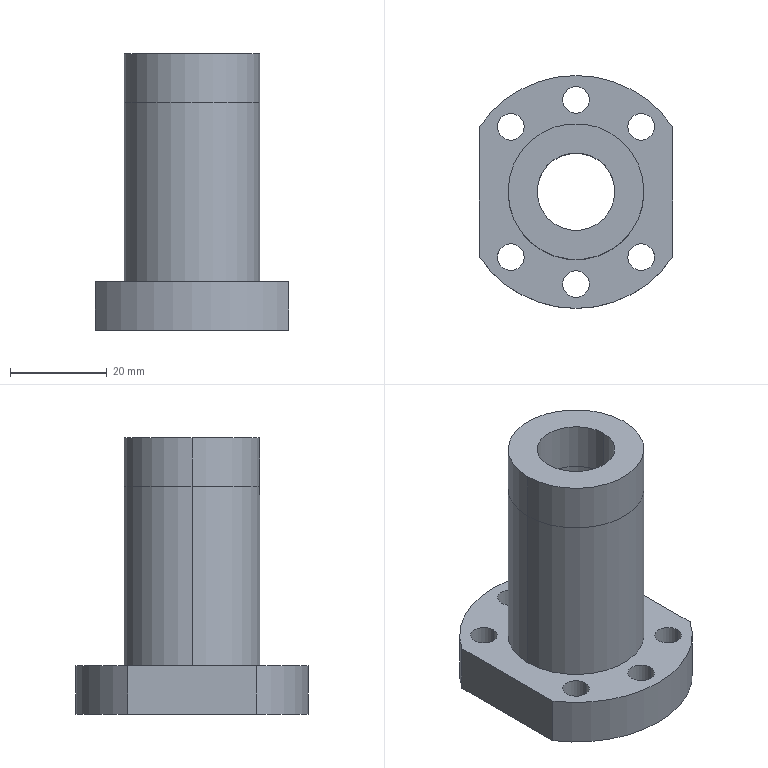Part | SolidWorks | features Extrusion 1, HoleWzd 1, ICE 1, MirrorPattern 1, Split 1 | 3 solids | 32 faces | box 40 x 48 x 57 mm | volume 32709 mm3 | cylinder 24 | plane 8 | commonest cylinder face diameters 5.5 x12 16 x6 28 x4 48 x2
STEP:
#1=CARTESIAN_POINT('',(-8.,0.,47.));
#2=VERTEX_POINT('',#1);
#3=CARTESIAN_POINT('',(8.,0.,47.));
#4=VERTEX_POINT('',#3);
#5=CARTESIAN_POINT('',(0.,0.,47.));
#6=DIRECTION('',(0.,0.,1.));
#7=DIRECTION('',(1.,0.,0.));
#8=AXIS2_PLACEMENT_3D('',#5,#6,#7);
#9=CIRCLE('',#8,8.);
#10=EDGE_CURVE('',#2,#4,#9,.T.);
#11=ORIENTED_EDGE('',*,*,#10,.T.);
#12=CARTESIAN_POINT('',(8.,0.,10.));
#13=VERTEX_POINT('',#12);
#14=CARTESIAN_POINT('',(8.,0.,57.));
#15=DIRECTION('',(0.,0.,-1.));
#16=VECTOR('',#15,1000.);
#17=LINE('',#14,#16);
#18=EDGE_CURVE('',#4,#13,#17,.T.);
#19=ORIENTED_EDGE('',*,*,#18,.T.);
#20=CARTESIAN_POINT('',(-8.,0.,10.));
#21=VERTEX_POINT('',#20);
#22=CARTESIAN_POINT('',(0.,0.,10.));
#23=DIRECTION('',(0.,0.,-1.));
#24=DIRECTION('',(-1.,0.,0.));
#25=AXIS2_PLACEMENT_3D('',#22,#23,#24);
#26=CIRCLE('',#25,8.);
#27=EDGE_CURVE('',#13,#21,#26,.T.);
#28=ORIENTED_EDGE('',*,*,#27,.T.);
#29=CARTESIAN_POINT('',(-8.,0.,57.));
#30=DIRECTION('',(0.,0.,-1.));
#31=VECTOR('',#30,1000.);
#32=LINE('',#29,#31);
#33=EDGE_CURVE('',#2,#21,#32,.T.);
#34=ORIENTED_EDGE('',*,*,#33,.F.);
#35=EDGE_LOOP('',(#11,#19,#28,#34));
#36=FACE_OUTER_BOUND('',#35,.T.);
#37=CARTESIAN_POINT('',(0.,0.,57.));
#38=DIRECTION('',(0.,0.,-1.));
#39=DIRECTION('',(-1.,0.,0.));
#40=AXIS2_PLACEMENT_3D('',#37,#38,#39);
#41=CYLINDRICAL_SURFACE('',#40,8.);
#42=ADVANCED_FACE('',(#36),#41,.F.);
#43=CARTESIAN_POINT('',(14.,0.,47.));
#44=VERTEX_POINT('',#43);
#45=CARTESIAN_POINT('',(-14.,0.,47.));
#46=VERTEX_POINT('',#45);
#47=CARTESIAN_POINT('',(0.,0.,47.));
#48=DIRECTION('',(0.,0.,1.));
#49=DIRECTION('',(1.,0.,0.));
#50=AXIS2_PLACEMENT_3D('',#47,#48,#49);
#51=CIRCLE('',#50,14.);
#52=EDGE_CURVE('',#44,#46,#51,.T.);
#53=ORIENTED_EDGE('',*,*,#52,.F.);
#54=CARTESIAN_POINT('',(14.,0.,10.));
#55=VERTEX_POINT('',#54);
#56=CARTESIAN_POINT('',(14.,0.,57.));
#57=DIRECTION('',(0.,0.,-1.));
#58=VECTOR('',#57,1000.);
#59=LINE('',#56,#58);
#60=EDGE_CURVE('',#44,#55,#59,.T.);
#61=ORIENTED_EDGE('',*,*,#60,.T.);
#62=CARTESIAN_POINT('',(-14.,0.,10.));
#63=VERTEX_POINT('',#62);
#64=CARTESIAN_POINT('',(0.,0.,10.));
#65=DIRECTION('',(0.,0.,-1.));
#66=DIRECTION('',(-1.,0.,0.));
#67=AXIS2_PLACEMENT_3D('',#64,#65,#66);
#68=CIRCLE('',#67,14.);
#69=EDGE_CURVE('',#63,#55,#68,.T.);
#70=ORIENTED_EDGE('',*,*,#69,.F.);
#71=CARTESIAN_POINT('',(-14.,0.,57.));
#72=DIRECTION('',(0.,0.,-1.));
#73=VECTOR('',#72,1000.);
#74=LINE('',#71,#73);
#75=EDGE_CURVE('',#46,#63,#74,.T.);
#76=ORIENTED_EDGE('',*,*,#75,.F.);
#77=EDGE_LOOP('',(#53,#61,#70,#76));
#78=FACE_OUTER_BOUND('',#77,.T.);
#79=CARTESIAN_POINT('',(0.,0.,57.));
#80=DIRECTION('',(0.,0.,-1.));
#81=DIRECTION('',(-1.,0.,0.));
#82=AXIS2_PLACEMENT_3D('',#79,#80,#81);
#83=CYLINDRICAL_SURFACE('',#82,14.);
#84=ADVANCED_FACE('',(#78),#83,.T.);
#85=ORIENTED_EDGE('',*,*,#60,.F.);
#86=CARTESIAN_POINT('',(0.,0.,47.));
#87=DIRECTION('',(0.,0.,1.));
#88=DIRECTION('',(1.,0.,0.));
#89=AXIS2_PLACEMENT_3D('',#86,#87,#88);
#90=CIRCLE('',#89,14.);
#91=EDGE_CURVE('',#46,#44,#90,.T.);
#92=ORIENTED_EDGE('',*,*,#91,.F.);
#93=ORIENTED_EDGE('',*,*,#75,.T.);
#94=CARTESIAN_POINT('',(0.,0.,10.));
#95=DIRECTION('',(0.,0.,-1.));
#96=DIRECTION('',(-1.,0.,0.));
#97=AXIS2_PLACEMENT_3D('',#94,#95,#96);
#98=CIRCLE('',#97,14.);
#99=EDGE_CURVE('',#55,#63,#98,.T.);
#100=ORIENTED_EDGE('',*,*,#99,.F.);
#101=EDGE_LOOP('',(#85,#92,#93,#100));
#102=FACE_OUTER_BOUND('',#101,.T.);
#103=CARTESIAN_POINT('',(0.,0.,57.));
#104=DIRECTION('',(0.,0.,-1.));
#105=DIRECTION('',(-1.,0.,0.));
#106=AXIS2_PLACEMENT_3D('',#103,#104,#105);
#107=CYLINDRICAL_SURFACE('',#106,14.);
#108=ADVANCED_FACE('',(#102),#107,.T.);
#109=ORIENTED_EDGE('',*,*,#18,.F.);
#110=CARTESIAN_POINT('',(0.,0.,47.));
#111=DIRECTION('',(0.,0.,1.));
#112=DIRECTION('',(1.,0.,0.));
#113=AXIS2_PLACEMENT_3D('',#110,#111,#112);
#114=CIRCLE('',#113,8.);
#115=EDGE_CURVE('',#4,#2,#114,.T.);
#116=ORIENTED_EDGE('',*,*,#115,.T.);
#117=ORIENTED_EDGE('',*,*,#33,.T.);
#118=CARTESIAN_POINT('',(0.,0.,10.));
#119=DIRECTION('',(0.,0.,-1.));
#120=DIRECTION('',(-1.,0.,0.));
#121=AXIS2_PLACEMENT_3D('',#118,#119,#120);
#122=CIRCLE('',#121,8.);
#123=EDGE_CURVE('',#21,#13,#122,.T.);
#124=ORIENTED_EDGE('',*,*,#123,.T.);
#125=EDGE_LOOP('',(#109,#116,#117,#124));
#126=FACE_OUTER_BOUND('',#125,.T.);
#127=CARTESIAN_POINT('',(0.,0.,57.));
#128=DIRECTION('',(0.,0.,-1.));
#129=DIRECTION('',(-1.,0.,0.));
#130=AXIS2_PLACEMENT_3D('',#127,#128,#129);
#131=CYLINDRICAL_SURFACE('',#130,8.);
#132=ADVANCED_FACE('',(#126),#131,.F.);
#133=ORIENTED_EDGE('',*,*,#91,.T.);
#134=ORIENTED_EDGE('',*,*,#52,.T.);
#135=EDGE_LOOP('',(#133,#134));
#136=FACE_OUTER_BOUND('',#135,.T.);
#137=ORIENTED_EDGE('',*,*,#10,.F.);
#138=ORIENTED_EDGE('',*,*,#115,.F.);
#139=EDGE_LOOP('',(#137,#138));
#140=FACE_BOUND('',#139,.T.);
#141=CARTESIAN_POINT('',(-26.149,-24.01,47.));
#142=DIRECTION('',(0.,0.,1.));
#143=DIRECTION('',(1.,0.,0.));
#144=AXIS2_PLACEMENT_3D('',#141,#142,#143);
#145=PLANE('',#144);
#146=ADVANCED_FACE('',(#136,#140),#145,.T.);
#147=ORIENTED_EDGE('',*,*,#69,.T.);
#148=ORIENTED_EDGE('',*,*,#99,.T.);
#149=EDGE_LOOP('',(#147,#148));
#150=FACE_OUTER_BOUND('',#149,.T.);
#151=ORIENTED_EDGE('',*,*,#123,.F.);
#152=ORIENTED_EDGE('',*,*,#27,.F.);
#153=EDGE_LOOP('',(#151,#152));
#154=FACE_BOUND('',#153,.T.);
#155=CARTESIAN_POINT('',(-26.149,-24.01,10.));
#156=DIRECTION('',(0.,0.,-1.));
#157=DIRECTION('',(-1.,0.,0.));
#158=AXIS2_PLACEMENT_3D('',#155,#156,#157);
#159=PLANE('',#158);
#160=ADVANCED_FACE('',(#150,#154),#159,.T.);
#161=CLOSED_SHELL('',(#42,#84,#108,#132,#146,#160));
#162=MANIFOLD_SOLID_BREP('',#161);
#163=CARTESIAN_POINT('',(8.,0.,10.));
#164=VERTEX_POINT('',#163);
#165=CARTESIAN_POINT('',(-8.,0.,10.));
#166=VERTEX_POINT('',#165);
#167=CARTESIAN_POINT('',(0.,0.,10.));
#168=DIRECTION('',(0.,0.,-1.));
#169=DIRECTION('',(-1.,0.,0.));
#170=AXIS2_PLACEMENT_3D('',#167,#168,#169);
#171=CIRCLE('',#170,8.);
#172=EDGE_CURVE('',#164,#166,#171,.T.);
#173=ORIENTED_EDGE('',*,*,#172,.F.);
#174=CARTESIAN_POINT('',(8.,0.,0.));
#175=VERTEX_POINT('',#174);
#176=CARTESIAN_POINT('',(8.,0.,57.));
#177=DIRECTION('',(0.,0.,-1.));
#178=VECTOR('',#177,1000.);
#179=LINE('',#176,#178);
#180=EDGE_CURVE('',#164,#175,#179,.T.);
#181=ORIENTED_EDGE('',*,*,#180,.T.);
#182=CARTESIAN_POINT('',(-8.,0.,0.));
#183=VERTEX_POINT('',#182);
#184=CARTESIAN_POINT('',(0.,0.,0.));
#185=DIRECTION('',(0.,0.,1.));
#186=DIRECTION('',(1.,0.,0.));
#187=AXIS2_PLACEMENT_3D('',#184,#185,#186);
#188=CIRCLE('',#187,8.);
#189=EDGE_CURVE('',#183,#175,#188,.T.);
#190=ORIENTED_EDGE('',*,*,#189,.F.);
#191=CARTESIAN_POINT('',(-8.,0.,57.));
#192=DIRECTION('',(0.,0.,-1.));
#193=VECTOR('',#192,1000.);
#194=LINE('',#191,#193);
#195=EDGE_CURVE('',#166,#183,#194,.T.);
#196=ORIENTED_EDGE('',*,*,#195,.F.);
#197=EDGE_LOOP('',(#173,#181,#190,#196));
#198=FACE_OUTER_BOUND('',#197,.T.);
#199=CARTESIAN_POINT('',(0.,0.,57.));
#200=DIRECTION('',(0.,0.,-1.));
#201=DIRECTION('',(-1.,0.,0.));
#202=AXIS2_PLACEMENT_3D('',#199,#200,#201);
#203=CYLINDRICAL_SURFACE('',#202,8.);
#204=ADVANCED_FACE('',(#198),#203,.F.);
#205=CARTESIAN_POINT('',(-10.685,13.435,10.));
#206=VERTEX_POINT('',#205);
#207=CARTESIAN_POINT('',(-16.185,13.435,10.));
#208=VERTEX_POINT('',#207);
#209=CARTESIAN_POINT('',(-13.435,13.435,10.));
#210=DIRECTION('',(0.,0.,-1.));
#211=DIRECTION('',(-1.,0.,0.));
#212=AXIS2_PLACEMENT_3D('',#209,#210,#211);
#213=CIRCLE('',#212,2.75);
#214=EDGE_CURVE('',#206,#208,#213,.T.);
#215=ORIENTED_EDGE('',*,*,#214,.F.);
#216=CARTESIAN_POINT('',(-10.685,13.435,0.));
#217=VERTEX_POINT('',#216);
#218=CARTESIAN_POINT('',(-10.685,13.435,0.));
#219=DIRECTION('',(0.,0.,-1.));
#220=VECTOR('',#219,1000.);
#221=LINE('',#218,#220);
#222=EDGE_CURVE('',#206,#217,#221,.T.);
#223=ORIENTED_EDGE('',*,*,#222,.T.);
#224=CARTESIAN_POINT('',(-16.185,13.435,0.));
#225=VERTEX_POINT('',#224);
#226=CARTESIAN_POINT('',(-13.435,13.435,0.));
#227=DIRECTION('',(0.,0.,-1.));
#228=DIRECTION('',(-1.,0.,0.));
#229=AXIS2_PLACEMENT_3D('',#226,#227,#228);
#230=CIRCLE('',#229,2.75);
#231=EDGE_CURVE('',#217,#225,#230,.T.);
#232=ORIENTED_EDGE('',*,*,#231,.T.);
#233=CARTESIAN_POINT('',(-16.185,13.435,0.));
#234=DIRECTION('',(0.,0.,-1.));
#235=VECTOR('',#234,1000.);
#236=LINE('',#233,#235);
#237=EDGE_CURVE('',#208,#225,#236,.T.);
#238=ORIENTED_EDGE('',*,*,#237,.F.);
#239=EDGE_LOOP('',(#215,#223,#232,#238));
#240=FACE_OUTER_BOUND('',#239,.T.);
#241=CARTESIAN_POINT('',(-13.435,13.435,0.));
#242=DIRECTION('',(0.,0.,-1.));
#243=DIRECTION('',(-1.,0.,0.));
#244=AXIS2_PLACEMENT_3D('',#241,#242,#243);
#245=CYLINDRICAL_SURFACE('',#244,2.75);
#246=ADVANCED_FACE('',(#240),#245,.F.);
#247=CARTESIAN_POINT('',(16.185,13.435,10.));
#248=VERTEX_POINT('',#247);
#249=CARTESIAN_POINT('',(10.685,13.435,10.));
#250=VERTEX_POINT('',#249);
#251=CARTESIAN_POINT('',(13.435,13.435,10.));
#252=DIRECTION('',(0.,0.,-1.));
#253=DIRECTION('',(-1.,0.,0.));
#254=AXIS2_PLACEMENT_3D('',#251,#252,#253);
#255=CIRCLE('',#254,2.75);
#256=EDGE_CURVE('',#248,#250,#255,.T.);
#257=ORIENTED_EDGE('',*,*,#256,.F.);
#258=CARTESIAN_POINT('',(16.185,13.435,0.));
#259=VERTEX_POINT('',#258);
#260=CARTESIAN_POINT('',(16.185,13.435,0.));
#261=DIRECTION('',(0.,0.,-1.));
#262=VECTOR('',#261,1000.);
#263=LINE('',#260,#262);
#264=EDGE_CURVE('',#248,#259,#263,.T.);
#265=ORIENTED_EDGE('',*,*,#264,.T.);
#266=CARTESIAN_POINT('',(10.685,13.435,0.));
#267=VERTEX_POINT('',#266);
#268=CARTESIAN_POINT('',(13.435,13.435,0.));
#269=DIRECTION('',(0.,0.,-1.));
#270=DIRECTION('',(-1.,0.,0.));
#271=AXIS2_PLACEMENT_3D('',#268,#269,#270);
#272=CIRCLE('',#271,2.75);
#273=EDGE_CURVE('',#259,#267,#272,.T.);
#274=ORIENTED_EDGE('',*,*,#273,.T.);
#275=CARTESIAN_POINT('',(10.685,13.435,0.));
#276=DIRECTION('',(0.,0.,-1.));
#277=VECTOR('',#276,1000.);
#278=LINE('',#275,#277);
#279=EDGE_CURVE('',#250,#267,#278,.T.);
#280=ORIENTED_EDGE('',*,*,#279,.F.);
#281=EDGE_LOOP('',(#257,#265,#274,#280));
#282=FACE_OUTER_BOUND('',#281,.T.);
#283=CARTESIAN_POINT('',(13.435,13.435,0.));
#284=DIRECTION('',(0.,0.,-1.));
#285=DIRECTION('',(-1.,0.,0.));
#286=AXIS2_PLACEMENT_3D('',#283,#284,#285);
#287=CYLINDRICAL_SURFACE('',#286,2.75);
#288=ADVANCED_FACE('',(#282),#287,.F.);
#289=CARTESIAN_POINT('',(2.75,19.,10.));
#290=VERTEX_POINT('',#289);
#291=CARTESIAN_POINT('',(-2.75,19.,10.));
#292=VERTEX_POINT('',#291);
#293=CARTESIAN_POINT('',(0.,19.,10.));
#294=DIRECTION('',(0.,0.,-1.));
#295=DIRECTION('',(-1.,0.,0.));
#296=AXIS2_PLACEMENT_3D('',#293,#294,#295);
#297=CIRCLE('',#296,2.75);
#298=EDGE_CURVE('',#290,#292,#297,.T.);
#299=ORIENTED_EDGE('',*,*,#298,.F.);
#300=CARTESIAN_POINT('',(2.75,19.,0.));
#301=VERTEX_POINT('',#300);
#302=CARTESIAN_POINT('',(2.75,19.,0.));
#303=DIRECTION('',(0.,0.,-1.));
#304=VECTOR('',#303,1000.);
#305=LINE('',#302,#304);
#306=EDGE_CURVE('',#290,#301,#305,.T.);
#307=ORIENTED_EDGE('',*,*,#306,.T.);
#308=CARTESIAN_POINT('',(-2.75,19.,0.));
#309=VERTEX_POINT('',#308);
#310=CARTESIAN_POINT('',(0.,19.,0.));
#311=DIRECTION('',(0.,0.,-1.));
#312=DIRECTION('',(-1.,0.,0.));
#313=AXIS2_PLACEMENT_3D('',#310,#311,#312);
#314=CIRCLE('',#313,2.75);
#315=EDGE_CURVE('',#301,#309,#314,.T.);
#316=ORIENTED_EDGE('',*,*,#315,.T.);
#317=CARTESIAN_POINT('',(-2.75,19.,0.));
#318=DIRECTION('',(0.,0.,-1.));
#319=VECTOR('',#318,1000.);
#320=LINE('',#317,#319);
#321=EDGE_CURVE('',#292,#309,#320,.T.);
#322=ORIENTED_EDGE('',*,*,#321,.F.);
#323=EDGE_LOOP('',(#299,#307,#316,#322));
#324=FACE_OUTER_BOUND('',#323,.T.);
#325=CARTESIAN_POINT('',(0.,19.,0.));
#326=DIRECTION('',(0.,0.,-1.));
#327=DIRECTION('',(-1.,0.,0.));
#328=AXIS2_PLACEMENT_3D('',#325,#326,#327);
#329=CYLINDRICAL_SURFACE('',#328,2.75);
#330=ADVANCED_FACE('',(#324),#329,.F.);
#331=CARTESIAN_POINT('',(-10.685,-13.435,10.));
#332=VERTEX_POINT('',#331);
#333=CARTESIAN_POINT('',(-16.185,-13.435,10.));
#334=VERTEX_POINT('',#333);
#335=CARTESIAN_POINT('',(-13.435,-13.435,10.));
#336=DIRECTION('',(0.,0.,-1.));
#337=DIRECTION('',(-1.,0.,0.));
#338=AXIS2_PLACEMENT_3D('',#335,#336,#337);
#339=CIRCLE('',#338,2.75);
#340=EDGE_CURVE('',#332,#334,#339,.T.);
#341=ORIENTED_EDGE('',*,*,#340,.F.);
#342=CARTESIAN_POINT('',(-10.685,-13.435,0.));
#343=VERTEX_POINT('',#342);
#344=CARTESIAN_POINT('',(-10.685,-13.435,0.));
#345=DIRECTION('',(0.,0.,-1.));
#346=VECTOR('',#345,1000.);
#347=LINE('',#344,#346);
#348=EDGE_CURVE('',#332,#343,#347,.T.);
#349=ORIENTED_EDGE('',*,*,#348,.T.);
#350=CARTESIAN_POINT('',(-16.185,-13.435,0.));
#351=VERTEX_POINT('',#350);
#352=CARTESIAN_POINT('',(-13.435,-13.435,0.));
#353=DIRECTION('',(0.,0.,-1.));
#354=DIRECTION('',(-1.,0.,0.));
#355=AXIS2_PLACEMENT_3D('',#352,#353,#354);
#356=CIRCLE('',#355,2.75);
#357=EDGE_CURVE('',#343,#351,#356,.T.);
#358=ORIENTED_EDGE('',*,*,#357,.T.);
#359=CARTESIAN_POINT('',(-16.185,-13.435,0.));
#360=DIRECTION('',(0.,0.,-1.));
#361=VECTOR('',#360,1000.);
#362=LINE('',#359,#361);
#363=EDGE_CURVE('',#334,#351,#362,.T.);
#364=ORIENTED_EDGE('',*,*,#363,.F.);
#365=EDGE_LOOP('',(#341,#349,#358,#364));
#366=FACE_OUTER_BOUND('',#365,.T.);
#367=CARTESIAN_POINT('',(-13.435,-13.435,0.));
#368=DIRECTION('',(0.,0.,-1.));
#369=DIRECTION('',(-1.,0.,0.));
#370=AXIS2_PLACEMENT_3D('',#367,#368,#369);
#371=CYLINDRICAL_SURFACE('',#370,2.75);
#372=ADVANCED_FACE('',(#366),#371,.F.);
#373=CARTESIAN_POINT('',(16.185,-13.435,10.));
#374=VERTEX_POINT('',#373);
#375=CARTESIAN_POINT('',(10.685,-13.435,10.));
#376=VERTEX_POINT('',#375);
#377=CARTESIAN_POINT('',(13.435,-13.435,10.));
#378=DIRECTION('',(0.,0.,-1.));
#379=DIRECTION('',(-1.,0.,0.));
#380=AXIS2_PLACEMENT_3D('',#377,#378,#379);
#381=CIRCLE('',#380,2.75);
#382=EDGE_CURVE('',#374,#376,#381,.T.);
#383=ORIENTED_EDGE('',*,*,#382,.F.);
#384=CARTESIAN_POINT('',(16.185,-13.435,0.));
#385=VERTEX_POINT('',#384);
#386=CARTESIAN_POINT('',(16.185,-13.435,0.));
#387=DIRECTION('',(0.,0.,-1.));
#388=VECTOR('',#387,1000.);
#389=LINE('',#386,#388);
#390=EDGE_CURVE('',#374,#385,#389,.T.);
#391=ORIENTED_EDGE('',*,*,#390,.T.);
#392=CARTESIAN_POINT('',(10.685,-13.435,0.));
#393=VERTEX_POINT('',#392);
#394=CARTESIAN_POINT('',(13.435,-13.435,0.));
#395=DIRECTION('',(0.,0.,-1.));
#396=DIRECTION('',(-1.,0.,0.));
#397=AXIS2_PLACEMENT_3D('',#394,#395,#396);
#398=CIRCLE('',#397,2.75);
#399=EDGE_CURVE('',#385,#393,#398,.T.);
#400=ORIENTED_EDGE('',*,*,#399,.T.);
#401=CARTESIAN_POINT('',(10.685,-13.435,0.));
#402=DIRECTION('',(0.,0.,-1.));
#403=VECTOR('',#402,1000.);
#404=LINE('',#401,#403);
#405=EDGE_CURVE('',#376,#393,#404,.T.);
#406=ORIENTED_EDGE('',*,*,#405,.F.);
#407=EDGE_LOOP('',(#383,#391,#400,#406));
#408=FACE_OUTER_BOUND('',#407,.T.);
#409=CARTESIAN_POINT('',(13.435,-13.435,0.));
#410=DIRECTION('',(0.,0.,-1.));
#411=DIRECTION('',(-1.,0.,0.));
#412=AXIS2_PLACEMENT_3D('',#409,#410,#411);
#413=CYLINDRICAL_SURFACE('',#412,2.75);
#414=ADVANCED_FACE('',(#408),#413,.F.);
#415=CARTESIAN_POINT('',(2.75,-19.,10.));
#416=VERTEX_POINT('',#415);
#417=CARTESIAN_POINT('',(-2.75,-19.,10.));
#418=VERTEX_POINT('',#417);
#419=CARTESIAN_POINT('',(0.,-19.,10.));
#420=DIRECTION('',(0.,0.,-1.));
#421=DIRECTION('',(-1.,0.,0.));
#422=AXIS2_PLACEMENT_3D('',#419,#420,#421);
#423=CIRCLE('',#422,2.75);
#424=EDGE_CURVE('',#416,#418,#423,.T.);
#425=ORIENTED_EDGE('',*,*,#424,.F.);
#426=CARTESIAN_POINT('',(2.75,-19.,0.));
#427=VERTEX_POINT('',#426);
#428=CARTESIAN_POINT('',(2.75,-19.,0.));
#429=DIRECTION('',(0.,0.,-1.));
#430=VECTOR('',#429,1000.);
#431=LINE('',#428,#430);
#432=EDGE_CURVE('',#416,#427,#431,.T.);
#433=ORIENTED_EDGE('',*,*,#432,.T.);
#434=CARTESIAN_POINT('',(-2.75,-19.,0.));
#435=VERTEX_POINT('',#434);
#436=CARTESIAN_POINT('',(0.,-19.,0.));
#437=DIRECTION('',(0.,0.,-1.));
#438=DIRECTION('',(-1.,0.,0.));
#439=AXIS2_PLACEMENT_3D('',#436,#437,#438);
#440=CIRCLE('',#439,2.75);
#441=EDGE_CURVE('',#427,#435,#440,.T.);
#442=ORIENTED_EDGE('',*,*,#441,.T.);
#443=CARTESIAN_POINT('',(-2.75,-19.,0.));
#444=DIRECTION('',(0.,0.,-1.));
#445=VECTOR('',#444,1000.);
#446=LINE('',#443,#445);
#447=EDGE_CURVE('',#418,#435,#446,.T.);
#448=ORIENTED_EDGE('',*,*,#447,.F.);
#449=EDGE_LOOP('',(#425,#433,#442,#448));
#450=FACE_OUTER_BOUND('',#449,.T.);
#451=CARTESIAN_POINT('',(0.,-19.,0.));
#452=DIRECTION('',(0.,0.,-1.));
#453=DIRECTION('',(-1.,0.,0.));
#454=AXIS2_PLACEMENT_3D('',#451,#452,#453);
#455=CYLINDRICAL_SURFACE('',#454,2.75);
#456=ADVANCED_FACE('',(#450),#455,.F.);
#457=ORIENTED_EDGE('',*,*,#180,.F.);
#458=CARTESIAN_POINT('',(0.,0.,10.));
#459=DIRECTION('',(0.,0.,-1.));
#460=DIRECTION('',(-1.,0.,0.));
#461=AXIS2_PLACEMENT_3D('',#458,#459,#460);
#462=CIRCLE('',#461,8.);
#463=EDGE_CURVE('',#166,#164,#462,.T.);
#464=ORIENTED_EDGE('',*,*,#463,.F.);
#465=ORIENTED_EDGE('',*,*,#195,.T.);
#466=CARTESIAN_POINT('',(0.,0.,0.));
#467=DIRECTION('',(0.,0.,1.));
#468=DIRECTION('',(1.,0.,0.));
#469=AXIS2_PLACEMENT_3D('',#466,#467,#468);
#470=CIRCLE('',#469,8.);
#471=EDGE_CURVE('',#175,#183,#470,.T.);
#472=ORIENTED_EDGE('',*,*,#471,.F.);
#473=EDGE_LOOP('',(#457,#464,#465,#472));
#474=FACE_OUTER_BOUND('',#473,.T.);
#475=CARTESIAN_POINT('',(0.,0.,57.));
#476=DIRECTION('',(0.,0.,-1.));
#477=DIRECTION('',(-1.,0.,0.));
#478=AXIS2_PLACEMENT_3D('',#475,#476,#477);
#479=CYLINDRICAL_SURFACE('',#478,8.);
#480=ADVANCED_FACE('',(#474),#479,.F.);
#481=CARTESIAN_POINT('',(-20.,13.266,0.));
#482=VERTEX_POINT('',#481);
#483=CARTESIAN_POINT('',(20.,13.266,0.));
#484=VERTEX_POINT('',#483);
#485=CARTESIAN_POINT('',(0.,0.,0.));
#486=DIRECTION('',(0.,0.,-1.));
#487=DIRECTION('',(-1.,0.,0.));
#488=AXIS2_PLACEMENT_3D('',#485,#486,#487);
#489=CIRCLE('',#488,24.);
#490=EDGE_CURVE('',#482,#484,#489,.T.);
#491=ORIENTED_EDGE('',*,*,#490,.F.);
#492=CARTESIAN_POINT('',(-20.,13.266,10.));
#493=VERTEX_POINT('',#492);
#494=CARTESIAN_POINT('',(-20.,13.266,10.));
#495=DIRECTION('',(0.,0.,-1.));
#496=VECTOR('',#495,1000.);
#497=LINE('',#494,#496);
#498=EDGE_CURVE('',#493,#482,#497,.T.);
#499=ORIENTED_EDGE('',*,*,#498,.F.);
#500=CARTESIAN_POINT('',(20.,13.266,10.));
#501=VERTEX_POINT('',#500);
#502=CARTESIAN_POINT('',(0.,0.,10.));
#503=DIRECTION('',(0.,0.,-1.));
#504=DIRECTION('',(-1.,0.,0.));
#505=AXIS2_PLACEMENT_3D('',#502,#503,#504);
#506=CIRCLE('',#505,24.);
#507=EDGE_CURVE('',#493,#501,#506,.T.);
#508=ORIENTED_EDGE('',*,*,#507,.T.);
#509=CARTESIAN_POINT('',(20.,13.266,10.));
#510=DIRECTION('',(0.,0.,-1.));
#511=VECTOR('',#510,1000.);
#512=LINE('',#509,#511);
#513=EDGE_CURVE('',#501,#484,#512,.T.);
#514=ORIENTED_EDGE('',*,*,#513,.T.);
#515=EDGE_LOOP('',(#491,#499,#508,#514));
#516=FACE_OUTER_BOUND('',#515,.T.);
#517=CARTESIAN_POINT('',(0.,0.,10.));
#518=DIRECTION('',(0.,0.,-1.));
#519=DIRECTION('',(-1.,0.,0.));
#520=AXIS2_PLACEMENT_3D('',#517,#518,#519);
#521=CYLINDRICAL_SURFACE('',#520,24.);
#522=ADVANCED_FACE('',(#516),#521,.T.);
#523=ORIENTED_EDGE('',*,*,#222,.F.);
#524=CARTESIAN_POINT('',(-13.435,13.435,10.));
#525=DIRECTION('',(0.,0.,-1.));
#526=DIRECTION('',(-1.,0.,0.));
#527=AXIS2_PLACEMENT_3D('',#524,#525,#526);
#528=CIRCLE('',#527,2.75);
#529=EDGE_CURVE('',#208,#206,#528,.T.);
#530=ORIENTED_EDGE('',*,*,#529,.F.);
#531=ORIENTED_EDGE('',*,*,#237,.T.);
#532=CARTESIAN_POINT('',(-13.435,13.435,0.));
#533=DIRECTION('',(0.,0.,-1.));
#534=DIRECTION('',(-1.,0.,0.));
#535=AXIS2_PLACEMENT_3D('',#532,#533,#534);
#536=CIRCLE('',#535,2.75);
#537=EDGE_CURVE('',#225,#217,#536,.T.);
#538=ORIENTED_EDGE('',*,*,#537,.T.);
#539=EDGE_LOOP('',(#523,#530,#531,#538));
#540=FACE_OUTER_BOUND('',#539,.T.);
#541=CARTESIAN_POINT('',(-13.435,13.435,0.));
#542=DIRECTION('',(0.,0.,-1.));
#543=DIRECTION('',(-1.,0.,0.));
#544=AXIS2_PLACEMENT_3D('',#541,#542,#543);
#545=CYLINDRICAL_SURFACE('',#544,2.75);
#546=ADVANCED_FACE('',(#540),#545,.F.);
#547=ORIENTED_EDGE('',*,*,#264,.F.);
#548=CARTESIAN_POINT('',(13.435,13.435,10.));
#549=DIRECTION('',(0.,0.,-1.));
#550=DIRECTION('',(-1.,0.,0.));
#551=AXIS2_PLACEMENT_3D('',#548,#549,#550);
#552=CIRCLE('',#551,2.75);
#553=EDGE_CURVE('',#250,#248,#552,.T.);
#554=ORIENTED_EDGE('',*,*,#553,.F.);
#555=ORIENTED_EDGE('',*,*,#279,.T.);
#556=CARTESIAN_POINT('',(13.435,13.435,0.));
#557=DIRECTION('',(0.,0.,-1.));
#558=DIRECTION('',(-1.,0.,0.));
#559=AXIS2_PLACEMENT_3D('',#556,#557,#558);
#560=CIRCLE('',#559,2.75);
#561=EDGE_CURVE('',#267,#259,#560,.T.);
#562=ORIENTED_EDGE('',*,*,#561,.T.);
#563=EDGE_LOOP('',(#547,#554,#555,#562));
#564=FACE_OUTER_BOUND('',#563,.T.);
#565=CARTESIAN_POINT('',(13.435,13.435,0.));
#566=DIRECTION('',(0.,0.,-1.));
#567=DIRECTION('',(-1.,0.,0.));
#568=AXIS2_PLACEMENT_3D('',#565,#566,#567);
#569=CYLINDRICAL_SURFACE('',#568,2.75);
#570=ADVANCED_FACE('',(#564),#569,.F.);
#571=ORIENTED_EDGE('',*,*,#306,.F.);
#572=CARTESIAN_POINT('',(0.,19.,10.));
#573=DIRECTION('',(0.,0.,-1.));
#574=DIRECTION('',(-1.,0.,0.));
#575=AXIS2_PLACEMENT_3D('',#572,#573,#574);
#576=CIRCLE('',#575,2.75);
#577=EDGE_CURVE('',#292,#290,#576,.T.);
#578=ORIENTED_EDGE('',*,*,#577,.F.);
#579=ORIENTED_EDGE('',*,*,#321,.T.);
#580=CARTESIAN_POINT('',(0.,19.,0.));
#581=DIRECTION('',(0.,0.,-1.));
#582=DIRECTION('',(-1.,0.,0.));
#583=AXIS2_PLACEMENT_3D('',#580,#581,#582);
#584=CIRCLE('',#583,2.75);
#585=EDGE_CURVE('',#309,#301,#584,.T.);
#586=ORIENTED_EDGE('',*,*,#585,.T.);
#587=EDGE_LOOP('',(#571,#578,#579,#586));
#588=FACE_OUTER_BOUND('',#587,.T.);
#589=CARTESIAN_POINT('',(0.,19.,0.));
#590=DIRECTION('',(0.,0.,-1.));
#591=DIRECTION('',(-1.,0.,0.));
#592=AXIS2_PLACEMENT_3D('',#589,#590,#591);
#593=CYLINDRICAL_SURFACE('',#592,2.75);
#594=ADVANCED_FACE('',(#588),#593,.F.);
#595=ORIENTED_EDGE('',*,*,#348,.F.);
#596=CARTESIAN_POINT('',(-13.435,-13.435,10.));
#597=DIRECTION('',(0.,0.,-1.));
#598=DIRECTION('',(-1.,0.,0.));
#599=AXIS2_PLACEMENT_3D('',#596,#597,#598);
#600=CIRCLE('',#599,2.75);
#601=EDGE_CURVE('',#334,#332,#600,.T.);
#602=ORIENTED_EDGE('',*,*,#601,.F.);
#603=ORIENTED_EDGE('',*,*,#363,.T.);
#604=CARTESIAN_POINT('',(-13.435,-13.435,0.));
#605=DIRECTION('',(0.,0.,-1.));
#606=DIRECTION('',(-1.,0.,0.));
#607=AXIS2_PLACEMENT_3D('',#604,#605,#606);
#608=CIRCLE('',#607,2.75);
#609=EDGE_CURVE('',#351,#343,#608,.T.);
#610=ORIENTED_EDGE('',*,*,#609,.T.);
#611=EDGE_LOOP('',(#595,#602,#603,#610));
#612=FACE_OUTER_BOUND('',#611,.T.);
#613=CARTESIAN_POINT('',(-13.435,-13.435,0.));
#614=DIRECTION('',(0.,0.,-1.));
#615=DIRECTION('',(-1.,0.,0.));
#616=AXIS2_PLACEMENT_3D('',#613,#614,#615);
#617=CYLINDRICAL_SURFACE('',#616,2.75);
#618=ADVANCED_FACE('',(#612),#617,.F.);
#619=ORIENTED_EDGE('',*,*,#390,.F.);
#620=CARTESIAN_POINT('',(13.435,-13.435,10.));
#621=DIRECTION('',(0.,0.,-1.));
#622=DIRECTION('',(-1.,0.,0.));
#623=AXIS2_PLACEMENT_3D('',#620,#621,#622);
#624=CIRCLE('',#623,2.75);
#625=EDGE_CURVE('',#376,#374,#624,.T.);
#626=ORIENTED_EDGE('',*,*,#625,.F.);
#627=ORIENTED_EDGE('',*,*,#405,.T.);
#628=CARTESIAN_POINT('',(13.435,-13.435,0.));
#629=DIRECTION('',(0.,0.,-1.));
#630=DIRECTION('',(-1.,0.,0.));
#631=AXIS2_PLACEMENT_3D('',#628,#629,#630);
#632=CIRCLE('',#631,2.75);
#633=EDGE_CURVE('',#393,#385,#632,.T.);
#634=ORIENTED_EDGE('',*,*,#633,.T.);
#635=EDGE_LOOP('',(#619,#626,#627,#634));
#636=FACE_OUTER_BOUND('',#635,.T.);
#637=CARTESIAN_POINT('',(13.435,-13.435,0.));
#638=DIRECTION('',(0.,0.,-1.));
#639=DIRECTION('',(-1.,0.,0.));
#640=AXIS2_PLACEMENT_3D('',#637,#638,#639);
#641=CYLINDRICAL_SURFACE('',#640,2.75);
#642=ADVANCED_FACE('',(#636),#641,.F.);
#643=ORIENTED_EDGE('',*,*,#432,.F.);
#644=CARTESIAN_POINT('',(0.,-19.,10.));
#645=DIRECTION('',(0.,0.,-1.));
#646=DIRECTION('',(-1.,0.,0.));
#647=AXIS2_PLACEMENT_3D('',#644,#645,#646);
#648=CIRCLE('',#647,2.75);
#649=EDGE_CURVE('',#418,#416,#648,.T.);
#650=ORIENTED_EDGE('',*,*,#649,.F.);
#651=ORIENTED_EDGE('',*,*,#447,.T.);
#652=CARTESIAN_POINT('',(0.,-19.,0.));
#653=DIRECTION('',(0.,0.,-1.));
#654=DIRECTION('',(-1.,0.,0.));
#655=AXIS2_PLACEMENT_3D('',#652,#653,#654);
#656=CIRCLE('',#655,2.75);
#657=EDGE_CURVE('',#435,#427,#656,.T.);
#658=ORIENTED_EDGE('',*,*,#657,.T.);
#659=EDGE_LOOP('',(#643,#650,#651,#658));
#660=FACE_OUTER_BOUND('',#659,.T.);
#661=CARTESIAN_POINT('',(0.,-19.,0.));
#662=DIRECTION('',(0.,0.,-1.));
#663=DIRECTION('',(-1.,0.,0.));
#664=AXIS2_PLACEMENT_3D('',#661,#662,#663);
#665=CYLINDRICAL_SURFACE('',#664,2.75);
#666=ADVANCED_FACE('',(#660),#665,.F.);
#667=ORIENTED_EDGE('',*,*,#657,.F.);
#668=ORIENTED_EDGE('',*,*,#441,.F.);
#669=EDGE_LOOP('',(#667,#668));
#670=FACE_BOUND('',#669,.T.);
#671=ORIENTED_EDGE('',*,*,#633,.F.);
#672=ORIENTED_EDGE('',*,*,#399,.F.);
#673=EDGE_LOOP('',(#671,#672));
#674=FACE_BOUND('',#673,.T.);
#675=CARTESIAN_POINT('',(-20.,-13.266,0.));
#676=VERTEX_POINT('',#675);
#677=CARTESIAN_POINT('',(-20.,-5.893,0.));
#678=DIRECTION('',(0.,-1.,0.));
#679=VECTOR('',#678,1000.);
#680=LINE('',#677,#679);
#681=EDGE_CURVE('',#482,#676,#680,.T.);
#682=ORIENTED_EDGE('',*,*,#681,.F.);
#683=ORIENTED_EDGE('',*,*,#490,.T.);
#684=CARTESIAN_POINT('',(20.,-13.266,0.));
#685=VERTEX_POINT('',#684);
#686=CARTESIAN_POINT('',(20.,-5.893,0.));
#687=DIRECTION('',(0.,-1.,0.));
#688=VECTOR('',#687,1000.);
#689=LINE('',#686,#688);
#690=EDGE_CURVE('',#484,#685,#689,.T.);
#691=ORIENTED_EDGE('',*,*,#690,.T.);
#692=CARTESIAN_POINT('',(0.,0.,0.));
#693=DIRECTION('',(0.,0.,-1.));
#694=DIRECTION('',(-1.,0.,0.));
#695=AXIS2_PLACEMENT_3D('',#692,#693,#694);
#696=CIRCLE('',#695,24.);
#697=EDGE_CURVE('',#685,#676,#696,.T.);
#698=ORIENTED_EDGE('',*,*,#697,.T.);
#699=EDGE_LOOP('',(#682,#683,#691,#698));
#700=FACE_OUTER_BOUND('',#699,.T.);
#701=ORIENTED_EDGE('',*,*,#189,.T.);
#702=ORIENTED_EDGE('',*,*,#471,.T.);
#703=EDGE_LOOP('',(#701,#702));
#704=FACE_BOUND('',#703,.T.);
#705=ORIENTED_EDGE('',*,*,#537,.F.);
#706=ORIENTED_EDGE('',*,*,#231,.F.);
#707=EDGE_LOOP('',(#705,#706));
#708=FACE_BOUND('',#707,.T.);
#709=ORIENTED_EDGE('',*,*,#561,.F.);
#710=ORIENTED_EDGE('',*,*,#273,.F.);
#711=EDGE_LOOP('',(#709,#710));
#712=FACE_BOUND('',#711,.T.);
#713=ORIENTED_EDGE('',*,*,#585,.F.);
#714=ORIENTED_EDGE('',*,*,#315,.F.);
#715=EDGE_LOOP('',(#713,#714));
#716=FACE_BOUND('',#715,.T.);
#717=ORIENTED_EDGE('',*,*,#609,.F.);
#718=ORIENTED_EDGE('',*,*,#357,.F.);
#719=EDGE_LOOP('',(#717,#718));
#720=FACE_BOUND('',#719,.T.);
#721=CARTESIAN_POINT('',(0.,0.,0.));
#722=DIRECTION('',(0.,0.,1.));
#723=DIRECTION('',(1.,0.,0.));
#724=AXIS2_PLACEMENT_3D('',#721,#722,#723);
#725=PLANE('',#724);
#726=ADVANCED_FACE('',(#670,#674,#700,#704,#708,#712,#716,#720),#725,.F.);
#727=ORIENTED_EDGE('',*,*,#681,.T.);
#728=CARTESIAN_POINT('',(-20.,-13.266,10.));
#729=VERTEX_POINT('',#728);
#730=CARTESIAN_POINT('',(-20.,-13.266,10.));
#731=DIRECTION('',(0.,0.,-1.));
#732=VECTOR('',#731,1000.);
#733=LINE('',#730,#732);
#734=EDGE_CURVE('',#729,#676,#733,.T.);
#735=ORIENTED_EDGE('',*,*,#734,.F.);
#736=CARTESIAN_POINT('',(-20.,-5.893,10.));
#737=DIRECTION('',(0.,-1.,0.));
#738=VECTOR('',#737,1000.);
#739=LINE('',#736,#738);
#740=EDGE_CURVE('',#493,#729,#739,.T.);
#741=ORIENTED_EDGE('',*,*,#740,.F.);
#742=ORIENTED_EDGE('',*,*,#498,.T.);
#743=EDGE_LOOP('',(#727,#735,#741,#742));
#744=FACE_OUTER_BOUND('',#743,.T.);
#745=CARTESIAN_POINT('',(-20.,-5.893,10.));
#746=DIRECTION('',(1.,0.,0.));
#747=DIRECTION('',(0.,1.,0.));
#748=AXIS2_PLACEMENT_3D('',#745,#746,#747);
#749=PLANE('',#748);
#750=ADVANCED_FACE('',(#744),#749,.F.);
#751=ORIENTED_EDGE('',*,*,#690,.F.);
#752=ORIENTED_EDGE('',*,*,#513,.F.);
#753=CARTESIAN_POINT('',(20.,-13.266,10.));
#754=VERTEX_POINT('',#753);
#755=CARTESIAN_POINT('',(20.,-5.893,10.));
#756=DIRECTION('',(0.,-1.,0.));
#757=VECTOR('',#756,1000.);
#758=LINE('',#755,#757);
#759=EDGE_CURVE('',#501,#754,#758,.T.);
#760=ORIENTED_EDGE('',*,*,#759,.T.);
#761=CARTESIAN_POINT('',(20.,-13.266,10.));
#762=DIRECTION('',(0.,0.,-1.));
#763=VECTOR('',#762,1000.);
#764=LINE('',#761,#763);
#765=EDGE_CURVE('',#754,#685,#764,.T.);
#766=ORIENTED_EDGE('',*,*,#765,.T.);
#767=EDGE_LOOP('',(#751,#752,#760,#766));
#768=FACE_OUTER_BOUND('',#767,.T.);
#769=CARTESIAN_POINT('',(20.,-5.893,10.));
#770=DIRECTION('',(1.,0.,0.));
#771=DIRECTION('',(0.,1.,0.));
#772=AXIS2_PLACEMENT_3D('',#769,#770,#771);
#773=PLANE('',#772);
#774=ADVANCED_FACE('',(#768),#773,.T.);
#775=ORIENTED_EDGE('',*,*,#697,.F.);
#776=ORIENTED_EDGE('',*,*,#765,.F.);
#777=CARTESIAN_POINT('',(0.,0.,10.));
#778=DIRECTION('',(0.,0.,-1.));
#779=DIRECTION('',(-1.,0.,0.));
#780=AXIS2_PLACEMENT_3D('',#777,#778,#779);
#781=CIRCLE('',#780,24.);
#782=EDGE_CURVE('',#754,#729,#781,.T.);
#783=ORIENTED_EDGE('',*,*,#782,.T.);
#784=ORIENTED_EDGE('',*,*,#734,.T.);
#785=EDGE_LOOP('',(#775,#776,#783,#784));
#786=FACE_OUTER_BOUND('',#785,.T.);
#787=CARTESIAN_POINT('',(0.,0.,10.));
#788=DIRECTION('',(0.,0.,-1.));
#789=DIRECTION('',(-1.,0.,0.));
#790=AXIS2_PLACEMENT_3D('',#787,#788,#789);
#791=CYLINDRICAL_SURFACE('',#790,24.);
#792=ADVANCED_FACE('',(#786),#791,.T.);
#793=ORIENTED_EDGE('',*,*,#649,.T.);
#794=ORIENTED_EDGE('',*,*,#424,.T.);
#795=EDGE_LOOP('',(#793,#794));
#796=FACE_BOUND('',#795,.T.);
#797=ORIENTED_EDGE('',*,*,#625,.T.);
#798=ORIENTED_EDGE('',*,*,#382,.T.);
#799=EDGE_LOOP('',(#797,#798));
#800=FACE_BOUND('',#799,.T.);
#801=ORIENTED_EDGE('',*,*,#601,.T.);
#802=ORIENTED_EDGE('',*,*,#340,.T.);
#803=EDGE_LOOP('',(#801,#802));
#804=FACE_BOUND('',#803,.T.);
#805=ORIENTED_EDGE('',*,*,#577,.T.);
#806=ORIENTED_EDGE('',*,*,#298,.T.);
#807=EDGE_LOOP('',(#805,#806));
#808=FACE_BOUND('',#807,.T.);
#809=ORIENTED_EDGE('',*,*,#553,.T.);
#810=ORIENTED_EDGE('',*,*,#256,.T.);
#811=EDGE_LOOP('',(#809,#810));
#812=FACE_BOUND('',#811,.T.);
#813=ORIENTED_EDGE('',*,*,#529,.T.);
#814=ORIENTED_EDGE('',*,*,#214,.T.);
#815=EDGE_LOOP('',(#813,#814));
#816=FACE_BOUND('',#815,.T.);
#817=ORIENTED_EDGE('',*,*,#740,.T.);
#818=ORIENTED_EDGE('',*,*,#782,.F.);
#819=ORIENTED_EDGE('',*,*,#759,.F.);
#820=ORIENTED_EDGE('',*,*,#507,.F.);
#821=EDGE_LOOP('',(#817,#818,#819,#820));
#822=FACE_OUTER_BOUND('',#821,.T.);
#823=ORIENTED_EDGE('',*,*,#463,.T.);
#824=ORIENTED_EDGE('',*,*,#172,.T.);
#825=EDGE_LOOP('',(#823,#824));
#826=FACE_BOUND('',#825,.T.);
#827=CARTESIAN_POINT('',(-71.46,-5.893,10.));
#828=DIRECTION('',(0.,0.,-1.));
#829=DIRECTION('',(-1.,0.,0.));
#830=AXIS2_PLACEMENT_3D('',#827,#828,#829);
#831=PLANE('',#830);
#832=ADVANCED_FACE('',(#796,#800,#804,#808,#812,#816,#822,#826),#831,.F.);
#833=CLOSED_SHELL('',(#204,#246,#288,#330,#372,#414,#456,#480,#522,#546,#570,#594,#618,#642,#666,#726,#750,#774,#792,#832));
#834=MANIFOLD_SOLID_BREP('',#833);
#835=CARTESIAN_POINT('',(14.,0.,57.));
#836=VERTEX_POINT('',#835);
#837=CARTESIAN_POINT('',(-14.,0.,57.));
#838=VERTEX_POINT('',#837);
#839=CARTESIAN_POINT('',(0.,0.,57.));
#840=DIRECTION('',(0.,0.,1.));
#841=DIRECTION('',(1.,0.,0.));
#842=AXIS2_PLACEMENT_3D('',#839,#840,#841);
#843=CIRCLE('',#842,14.);
#844=EDGE_CURVE('',#836,#838,#843,.T.);
#845=ORIENTED_EDGE('',*,*,#844,.F.);
#846=CARTESIAN_POINT('',(14.,0.,47.));
#847=VERTEX_POINT('',#846);
#848=CARTESIAN_POINT('',(14.,0.,57.));
#849=DIRECTION('',(0.,0.,-1.));
#850=VECTOR('',#849,1000.);
#851=LINE('',#848,#850);
#852=EDGE_CURVE('',#836,#847,#851,.T.);
#853=ORIENTED_EDGE('',*,*,#852,.T.);
#854=CARTESIAN_POINT('',(-14.,0.,47.));
#855=VERTEX_POINT('',#854);
#856=CARTESIAN_POINT('',(0.,0.,47.));
#857=DIRECTION('',(0.,0.,1.));
#858=DIRECTION('',(1.,0.,0.));
#859=AXIS2_PLACEMENT_3D('',#856,#857,#858);
#860=CIRCLE('',#859,14.);
#861=EDGE_CURVE('',#847,#855,#860,.T.);
#862=ORIENTED_EDGE('',*,*,#861,.T.);
#863=CARTESIAN_POINT('',(-14.,0.,57.));
#864=DIRECTION('',(0.,0.,-1.));
#865=VECTOR('',#864,1000.);
#866=LINE('',#863,#865);
#867=EDGE_CURVE('',#838,#855,#866,.T.);
#868=ORIENTED_EDGE('',*,*,#867,.F.);
#869=EDGE_LOOP('',(#845,#853,#862,#868));
#870=FACE_OUTER_BOUND('',#869,.T.);
#871=CARTESIAN_POINT('',(0.,0.,57.));
#872=DIRECTION('',(0.,0.,-1.));
#873=DIRECTION('',(-1.,0.,0.));
#874=AXIS2_PLACEMENT_3D('',#871,#872,#873);
#875=CYLINDRICAL_SURFACE('',#874,14.);
#876=ADVANCED_FACE('',(#870),#875,.T.);
#877=CARTESIAN_POINT('',(-8.,0.,57.));
#878=VERTEX_POINT('',#877);
#879=CARTESIAN_POINT('',(8.,0.,57.));
#880=VERTEX_POINT('',#879);
#881=CARTESIAN_POINT('',(0.,0.,57.));
#882=DIRECTION('',(0.,0.,1.));
#883=DIRECTION('',(1.,0.,0.));
#884=AXIS2_PLACEMENT_3D('',#881,#882,#883);
#885=CIRCLE('',#884,8.);
#886=EDGE_CURVE('',#878,#880,#885,.T.);
#887=ORIENTED_EDGE('',*,*,#886,.T.);
#888=CARTESIAN_POINT('',(8.,0.,47.));
#889=VERTEX_POINT('',#888);
#890=CARTESIAN_POINT('',(8.,0.,57.));
#891=DIRECTION('',(0.,0.,-1.));
#892=VECTOR('',#891,1000.);
#893=LINE('',#890,#892);
#894=EDGE_CURVE('',#880,#889,#893,.T.);
#895=ORIENTED_EDGE('',*,*,#894,.T.);
#896=CARTESIAN_POINT('',(-8.,0.,47.));
#897=VERTEX_POINT('',#896);
#898=CARTESIAN_POINT('',(0.,0.,47.));
#899=DIRECTION('',(0.,0.,1.));
#900=DIRECTION('',(1.,0.,0.));
#901=AXIS2_PLACEMENT_3D('',#898,#899,#900);
#902=CIRCLE('',#901,8.);
#903=EDGE_CURVE('',#897,#889,#902,.T.);
#904=ORIENTED_EDGE('',*,*,#903,.F.);
#905=CARTESIAN_POINT('',(-8.,0.,57.));
#906=DIRECTION('',(0.,0.,-1.));
#907=VECTOR('',#906,1000.);
#908=LINE('',#905,#907);
#909=EDGE_CURVE('',#878,#897,#908,.T.);
#910=ORIENTED_EDGE('',*,*,#909,.F.);
#911=EDGE_LOOP('',(#887,#895,#904,#910));
#912=FACE_OUTER_BOUND('',#911,.T.);
#913=CARTESIAN_POINT('',(0.,0.,57.));
#914=DIRECTION('',(0.,0.,-1.));
#915=DIRECTION('',(-1.,0.,0.));
#916=AXIS2_PLACEMENT_3D('',#913,#914,#915);
#917=CYLINDRICAL_SURFACE('',#916,8.);
#918=ADVANCED_FACE('',(#912),#917,.F.);
#919=ORIENTED_EDGE('',*,*,#903,.T.);
#920=CARTESIAN_POINT('',(0.,0.,47.));
#921=DIRECTION('',(0.,0.,1.));
#922=DIRECTION('',(1.,0.,0.));
#923=AXIS2_PLACEMENT_3D('',#920,#921,#922);
#924=CIRCLE('',#923,8.);
#925=EDGE_CURVE('',#889,#897,#924,.T.);
#926=ORIENTED_EDGE('',*,*,#925,.T.);
#927=EDGE_LOOP('',(#919,#926));
#928=FACE_BOUND('',#927,.T.);
#929=CARTESIAN_POINT('',(0.,0.,47.));
#930=DIRECTION('',(0.,0.,1.));
#931=DIRECTION('',(1.,0.,0.));
#932=AXIS2_PLACEMENT_3D('',#929,#930,#931);
#933=CIRCLE('',#932,14.);
#934=EDGE_CURVE('',#855,#847,#933,.T.);
#935=ORIENTED_EDGE('',*,*,#934,.F.);
#936=ORIENTED_EDGE('',*,*,#861,.F.);
#937=EDGE_LOOP('',(#935,#936));
#938=FACE_OUTER_BOUND('',#937,.T.);
#939=CARTESIAN_POINT('',(-26.149,-24.01,47.));
#940=DIRECTION('',(0.,0.,1.));
#941=DIRECTION('',(1.,0.,0.));
#942=AXIS2_PLACEMENT_3D('',#939,#940,#941);
#943=PLANE('',#942);
#944=ADVANCED_FACE('',(#928,#938),#943,.F.);
#945=CARTESIAN_POINT('',(0.,0.,57.));
#946=DIRECTION('',(0.,0.,1.));
#947=DIRECTION('',(1.,0.,0.));
#948=AXIS2_PLACEMENT_3D('',#945,#946,#947);
#949=CIRCLE('',#948,14.);
#950=EDGE_CURVE('',#838,#836,#949,.T.);
#951=ORIENTED_EDGE('',*,*,#950,.T.);
#952=ORIENTED_EDGE('',*,*,#844,.T.);
#953=EDGE_LOOP('',(#951,#952));
#954=FACE_OUTER_BOUND('',#953,.T.);
#955=ORIENTED_EDGE('',*,*,#886,.F.);
#956=CARTESIAN_POINT('',(0.,0.,57.));
#957=DIRECTION('',(0.,0.,1.));
#958=DIRECTION('',(1.,0.,0.));
#959=AXIS2_PLACEMENT_3D('',#956,#957,#958);
#960=CIRCLE('',#959,8.);
#961=EDGE_CURVE('',#880,#878,#960,.T.);
#962=ORIENTED_EDGE('',*,*,#961,.F.);
#963=EDGE_LOOP('',(#955,#962));
#964=FACE_BOUND('',#963,.T.);
#965=CARTESIAN_POINT('',(0.,0.,57.));
#966=DIRECTION('',(0.,0.,1.));
#967=DIRECTION('',(1.,0.,0.));
#968=AXIS2_PLACEMENT_3D('',#965,#966,#967);
#969=PLANE('',#968);
#970=ADVANCED_FACE('',(#954,#964),#969,.T.);
#971=ORIENTED_EDGE('',*,*,#852,.F.);
#972=ORIENTED_EDGE('',*,*,#950,.F.);
#973=ORIENTED_EDGE('',*,*,#867,.T.);
#974=ORIENTED_EDGE('',*,*,#934,.T.);
#975=EDGE_LOOP('',(#971,#972,#973,#974));
#976=FACE_OUTER_BOUND('',#975,.T.);
#977=CARTESIAN_POINT('',(0.,0.,57.));
#978=DIRECTION('',(0.,0.,-1.));
#979=DIRECTION('',(-1.,0.,0.));
#980=AXIS2_PLACEMENT_3D('',#977,#978,#979);
#981=CYLINDRICAL_SURFACE('',#980,14.);
#982=ADVANCED_FACE('',(#976),#981,.T.);
#983=ORIENTED_EDGE('',*,*,#894,.F.);
#984=ORIENTED_EDGE('',*,*,#961,.T.);
#985=ORIENTED_EDGE('',*,*,#909,.T.);
#986=ORIENTED_EDGE('',*,*,#925,.F.);
#987=EDGE_LOOP('',(#983,#984,#985,#986));
#988=FACE_OUTER_BOUND('',#987,.T.);
#989=CARTESIAN_POINT('',(0.,0.,57.));
#990=DIRECTION('',(0.,0.,-1.));
#991=DIRECTION('',(-1.,0.,0.));
#992=AXIS2_PLACEMENT_3D('',#989,#990,#991);
#993=CYLINDRICAL_SURFACE('',#992,8.);
#994=ADVANCED_FACE('',(#988),#993,.F.);
#995=CLOSED_SHELL('',(#876,#918,#944,#970,#982,#994));
#996=MANIFOLD_SOLID_BREP('',#995);
#997=CARTESIAN_POINT('',(0.,0.,0.));
#998=DIRECTION('',(0.,0.,1.));
#999=DIRECTION('',(1.,0.,0.));
#1000=AXIS2_PLACEMENT_3D('',#997,#998,#999);
#1001=(LENGTH_UNIT()NAMED_UNIT(*)SI_UNIT(.MILLI.,.METRE.));
#1002=UNCERTAINTY_MEASURE_WITH_UNIT(LENGTH_MEASURE(0.00001),#1001,'','');
#1003=(NAMED_UNIT(*)PLANE_ANGLE_UNIT()SI_UNIT($,.RADIAN.));
#1004=(NAMED_UNIT(*)SI_UNIT($,.STERADIAN.)SOLID_ANGLE_UNIT());
#1005=(GEOMETRIC_REPRESENTATION_CONTEXT(3)GLOBAL_UNCERTAINTY_ASSIGNED_CONTEXT((#1002))GLOBAL_UNIT_ASSIGNED_CONTEXT((#1001,#1003,#1004))REPRESENTATION_CONTEXT('',''));
#1006=ADVANCED_BREP_SHAPE_REPRESENTATION('',(#162,#834,#996,#1000),#1005);